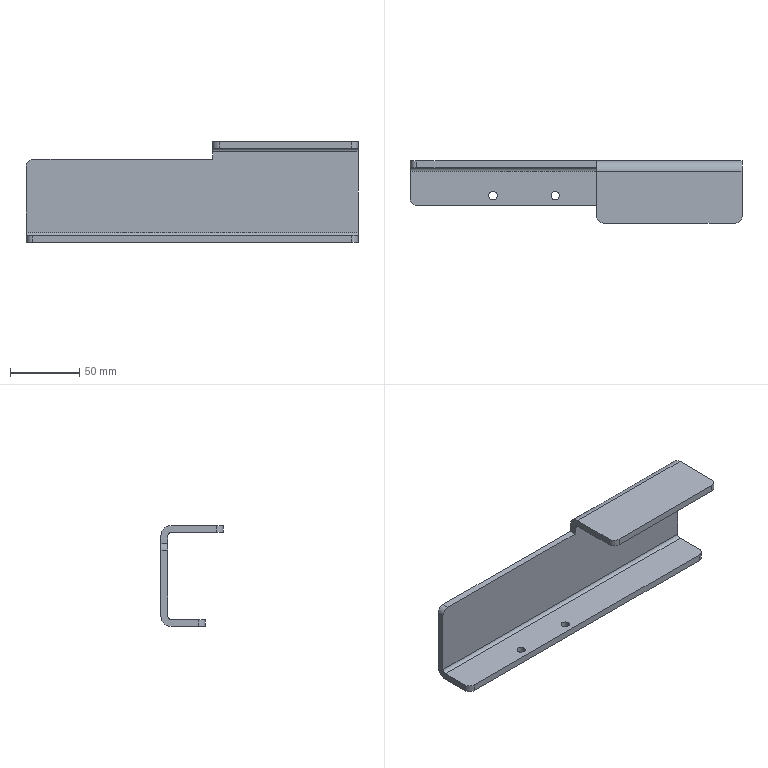Part | NX | 1 solid | 29 faces | box 240 x 45 x 73 mm | volume 128180 mm3 | cylinder 13 | plane 12 | cone 4 | commonest cylinder face diameters 10 x5 6 x4 4.8 x2 14.8 x2
STEP:
#1=CARTESIAN_POINT('',(2327.5,238.4,-44.7));
#2=VERTEX_POINT('',#1);
#3=CARTESIAN_POINT('',(2327.5,238.4,-49.7));
#4=VERTEX_POINT('',#3);
#5=CARTESIAN_POINT('',(2327.5,238.4,-49.7));
#6=DIRECTION('',(0.,0.,-1.));
#7=VECTOR('',#6,1000.);
#8=LINE('',#5,#7);
#9=EDGE_CURVE('',#2,#4,#8,.T.);
#10=ORIENTED_EDGE('',*,*,#9,.F.);
#11=CARTESIAN_POINT('',(2097.5,238.4,-44.7));
#12=VERTEX_POINT('',#11);
#13=CARTESIAN_POINT('',(2161.418,238.4,-44.7));
#14=DIRECTION('',(-1.,0.,0.));
#15=VECTOR('',#14,1000.);
#16=LINE('',#13,#15);
#17=EDGE_CURVE('',#2,#12,#16,.T.);
#18=ORIENTED_EDGE('',*,*,#17,.T.);
#19=CARTESIAN_POINT('',(2097.5,238.4,-49.7));
#20=VERTEX_POINT('',#19);
#21=CARTESIAN_POINT('',(2097.5,238.4,-49.7));
#22=DIRECTION('',(0.,0.,1.));
#23=VECTOR('',#22,1000.);
#24=LINE('',#21,#23);
#25=EDGE_CURVE('',#20,#12,#24,.T.);
#26=ORIENTED_EDGE('',*,*,#25,.F.);
#27=CARTESIAN_POINT('',(2161.418,238.4,-49.7));
#28=DIRECTION('',(-1.,0.,0.));
#29=VECTOR('',#28,1000.);
#30=LINE('',#27,#29);
#31=EDGE_CURVE('',#4,#20,#30,.T.);
#32=ORIENTED_EDGE('',*,*,#31,.F.);
#33=EDGE_LOOP('',(#10,#18,#26,#32));
#34=FACE_BOUND('',#33,.T.);
#35=CARTESIAN_POINT('',(2227.5,238.4,-49.7));
#36=DIRECTION('',(0.,-1.,0.));
#37=DIRECTION('',(0.,0.,-1.));
#38=AXIS2_PLACEMENT_3D('',#35,#36,#37);
#39=PLANE('',#38);
#40=ADVANCED_FACE('',(#34),#39,.T.);
#41=ORIENTED_EDGE('',*,*,#9,.T.);
#42=CARTESIAN_POINT('',(2332.5,243.4,-49.7));
#43=VERTEX_POINT('',#42);
#44=CARTESIAN_POINT('',(2327.5,243.4,-49.7));
#45=DIRECTION('',(0.,0.,-1.));
#46=DIRECTION('',(-1.,0.,0.));
#47=AXIS2_PLACEMENT_3D('',#44,#45,#46);
#48=CIRCLE('',#47,5.);
#49=EDGE_CURVE('',#43,#4,#48,.T.);
#50=ORIENTED_EDGE('',*,*,#49,.F.);
#51=CARTESIAN_POINT('',(2332.5,243.4,-44.7));
#52=VERTEX_POINT('',#51);
#53=CARTESIAN_POINT('',(2332.5,243.4,-49.7));
#54=DIRECTION('',(0.,0.,-1.));
#55=VECTOR('',#54,1000.);
#56=LINE('',#53,#55);
#57=EDGE_CURVE('',#52,#43,#56,.T.);
#58=ORIENTED_EDGE('',*,*,#57,.F.);
#59=CARTESIAN_POINT('',(2327.5,243.4,-44.7));
#60=DIRECTION('',(0.,0.,-1.));
#61=DIRECTION('',(-1.,0.,0.));
#62=AXIS2_PLACEMENT_3D('',#59,#60,#61);
#63=CIRCLE('',#62,5.);
#64=EDGE_CURVE('',#52,#2,#63,.T.);
#65=ORIENTED_EDGE('',*,*,#64,.T.);
#66=EDGE_LOOP('',(#41,#50,#58,#65));
#67=FACE_BOUND('',#66,.T.);
#68=CARTESIAN_POINT('',(2327.5,243.4,-49.7));
#69=DIRECTION('',(0.,0.,-1.));
#70=DIRECTION('',(-1.,0.,0.));
#71=AXIS2_PLACEMENT_3D('',#68,#69,#70);
#72=CYLINDRICAL_SURFACE('',#71,5.);
#73=ADVANCED_FACE('',(#67),#72,.T.);
#74=CARTESIAN_POINT('',(2200.5,245.4,-49.5));
#75=VERTEX_POINT('',#74);
#76=CARTESIAN_POINT('',(2194.5,245.4,-49.5));
#77=VERTEX_POINT('',#76);
#78=CARTESIAN_POINT('',(2197.5,245.4,-49.5));
#79=DIRECTION('',(0.,0.,-1.));
#80=DIRECTION('',(-1.,0.,0.));
#81=AXIS2_PLACEMENT_3D('',#78,#79,#80);
#82=CIRCLE('',#81,3.);
#83=EDGE_CURVE('',#75,#77,#82,.T.);
#84=ORIENTED_EDGE('',*,*,#83,.T.);
#85=CARTESIAN_POINT('',(2194.5,245.4,-44.7));
#86=VERTEX_POINT('',#85);
#87=CARTESIAN_POINT('',(2194.5,245.4,-49.7));
#88=DIRECTION('',(0.,0.,-1.));
#89=VECTOR('',#88,1000.);
#90=LINE('',#87,#89);
#91=EDGE_CURVE('',#77,#86,#90,.F.);
#92=ORIENTED_EDGE('',*,*,#91,.T.);
#93=CARTESIAN_POINT('',(2200.5,245.4,-44.7));
#94=VERTEX_POINT('',#93);
#95=CARTESIAN_POINT('',(2197.5,245.4,-44.7));
#96=DIRECTION('',(0.,0.,-1.));
#97=DIRECTION('',(-1.,0.,0.));
#98=AXIS2_PLACEMENT_3D('',#95,#96,#97);
#99=CIRCLE('',#98,3.);
#100=EDGE_CURVE('',#94,#86,#99,.T.);
#101=ORIENTED_EDGE('',*,*,#100,.F.);
#102=CARTESIAN_POINT('',(2200.5,245.4,-49.7));
#103=DIRECTION('',(0.,0.,-1.));
#104=VECTOR('',#103,1000.);
#105=LINE('',#102,#104);
#106=EDGE_CURVE('',#75,#94,#105,.F.);
#107=ORIENTED_EDGE('',*,*,#106,.F.);
#108=EDGE_LOOP('',(#84,#92,#101,#107));
#109=FACE_BOUND('',#108,.T.);
#110=CARTESIAN_POINT('',(2197.5,245.4,-49.7));
#111=DIRECTION('',(0.,0.,-1.));
#112=DIRECTION('',(-1.,0.,0.));
#113=AXIS2_PLACEMENT_3D('',#110,#111,#112);
#114=CYLINDRICAL_SURFACE('',#113,3.);
#115=ADVANCED_FACE('',(#109),#114,.F.);
#116=ORIENTED_EDGE('',*,*,#83,.F.);
#117=CARTESIAN_POINT('',(2200.7,245.4,-49.7));
#118=VERTEX_POINT('',#117);
#119=CARTESIAN_POINT('',(2200.5,245.4,-49.5));
#120=DIRECTION('',(0.7071,0.,-0.7071));
#121=VECTOR('',#120,1000.);
#122=LINE('',#119,#121);
#123=EDGE_CURVE('',#118,#75,#122,.F.);
#124=ORIENTED_EDGE('',*,*,#123,.F.);
#125=CARTESIAN_POINT('',(2194.3,245.4,-49.7));
#126=VERTEX_POINT('',#125);
#127=CARTESIAN_POINT('',(2197.5,245.4,-49.7));
#128=DIRECTION('',(0.,0.,-1.));
#129=DIRECTION('',(-1.,0.,0.));
#130=AXIS2_PLACEMENT_3D('',#127,#128,#129);
#131=CIRCLE('',#130,3.2);
#132=EDGE_CURVE('',#118,#126,#131,.T.);
#133=ORIENTED_EDGE('',*,*,#132,.T.);
#134=CARTESIAN_POINT('',(2194.5,245.4,-49.5));
#135=DIRECTION('',(-0.7071,0.,-0.7071));
#136=VECTOR('',#135,1000.);
#137=LINE('',#134,#136);
#138=EDGE_CURVE('',#126,#77,#137,.F.);
#139=ORIENTED_EDGE('',*,*,#138,.T.);
#140=EDGE_LOOP('',(#116,#124,#133,#139));
#141=FACE_BOUND('',#140,.T.);
#142=CARTESIAN_POINT('',(2197.5,245.4,-49.5));
#143=DIRECTION('',(0.,0.,-1.));
#144=DIRECTION('',(-1.,0.,0.));
#145=AXIS2_PLACEMENT_3D('',#142,#143,#144);
#146=CONICAL_SURFACE('',#145,3.,0.7854);
#147=ADVANCED_FACE('',(#141),#146,.F.);
#148=ORIENTED_EDGE('',*,*,#91,.F.);
#149=CARTESIAN_POINT('',(2197.5,245.4,-49.5));
#150=DIRECTION('',(0.,0.,-1.));
#151=DIRECTION('',(-1.,0.,0.));
#152=AXIS2_PLACEMENT_3D('',#149,#150,#151);
#153=CIRCLE('',#152,3.);
#154=EDGE_CURVE('',#77,#75,#153,.T.);
#155=ORIENTED_EDGE('',*,*,#154,.T.);
#156=ORIENTED_EDGE('',*,*,#106,.T.);
#157=CARTESIAN_POINT('',(2197.5,245.4,-44.7));
#158=DIRECTION('',(0.,0.,-1.));
#159=DIRECTION('',(-1.,0.,0.));
#160=AXIS2_PLACEMENT_3D('',#157,#158,#159);
#161=CIRCLE('',#160,3.);
#162=EDGE_CURVE('',#86,#94,#161,.T.);
#163=ORIENTED_EDGE('',*,*,#162,.F.);
#164=EDGE_LOOP('',(#148,#155,#156,#163));
#165=FACE_BOUND('',#164,.T.);
#166=CARTESIAN_POINT('',(2197.5,245.4,-49.7));
#167=DIRECTION('',(0.,0.,-1.));
#168=DIRECTION('',(-1.,0.,0.));
#169=AXIS2_PLACEMENT_3D('',#166,#167,#168);
#170=CYLINDRICAL_SURFACE('',#169,3.);
#171=ADVANCED_FACE('',(#165),#170,.F.);
#172=ORIENTED_EDGE('',*,*,#138,.F.);
#173=CARTESIAN_POINT('',(2197.5,245.4,-49.7));
#174=DIRECTION('',(0.,0.,-1.));
#175=DIRECTION('',(-1.,0.,0.));
#176=AXIS2_PLACEMENT_3D('',#173,#174,#175);
#177=CIRCLE('',#176,3.2);
#178=EDGE_CURVE('',#126,#118,#177,.T.);
#179=ORIENTED_EDGE('',*,*,#178,.T.);
#180=ORIENTED_EDGE('',*,*,#123,.T.);
#181=ORIENTED_EDGE('',*,*,#154,.F.);
#182=EDGE_LOOP('',(#172,#179,#180,#181));
#183=FACE_BOUND('',#182,.T.);
#184=CARTESIAN_POINT('',(2197.5,245.4,-49.5));
#185=DIRECTION('',(0.,0.,-1.));
#186=DIRECTION('',(-1.,0.,0.));
#187=AXIS2_PLACEMENT_3D('',#184,#185,#186);
#188=CONICAL_SURFACE('',#187,3.,0.7854);
#189=ADVANCED_FACE('',(#183),#188,.F.);
#190=CARTESIAN_POINT('',(2092.5,263.,-44.7));
#191=VERTEX_POINT('',#190);
#192=CARTESIAN_POINT('',(2092.5,243.4,-44.7));
#193=VERTEX_POINT('',#192);
#194=CARTESIAN_POINT('',(2092.5,301.297,-44.7));
#195=DIRECTION('',(0.,-1.,0.));
#196=VECTOR('',#195,1000.);
#197=LINE('',#194,#196);
#198=EDGE_CURVE('',#191,#193,#197,.T.);
#199=ORIENTED_EDGE('',*,*,#198,.T.);
#200=CARTESIAN_POINT('',(2097.5,243.4,-44.7));
#201=DIRECTION('',(0.,0.,1.));
#202=DIRECTION('',(1.,0.,0.));
#203=AXIS2_PLACEMENT_3D('',#200,#201,#202);
#204=CIRCLE('',#203,5.);
#205=EDGE_CURVE('',#193,#12,#204,.T.);
#206=ORIENTED_EDGE('',*,*,#205,.T.);
#207=ORIENTED_EDGE('',*,*,#17,.F.);
#208=ORIENTED_EDGE('',*,*,#64,.F.);
#209=CARTESIAN_POINT('',(2332.5,263.,-44.7));
#210=VERTEX_POINT('',#209);
#211=CARTESIAN_POINT('',(2332.5,249.699,-44.7));
#212=DIRECTION('',(0.,1.,0.));
#213=VECTOR('',#212,1000.);
#214=LINE('',#211,#213);
#215=EDGE_CURVE('',#52,#210,#214,.T.);
#216=ORIENTED_EDGE('',*,*,#215,.T.);
#217=CARTESIAN_POINT('',(2161.418,263.,-44.7));
#218=DIRECTION('',(-1.,0.,0.));
#219=VECTOR('',#218,1000.);
#220=LINE('',#217,#219);
#221=EDGE_CURVE('',#210,#191,#220,.T.);
#222=ORIENTED_EDGE('',*,*,#221,.T.);
#223=EDGE_LOOP('',(#199,#206,#207,#208,#216,#222));
#224=FACE_BOUND('',#223,.T.);
#225=CARTESIAN_POINT('',(2155.5,245.4,-44.7));
#226=VERTEX_POINT('',#225);
#227=CARTESIAN_POINT('',(2149.5,245.4,-44.7));
#228=VERTEX_POINT('',#227);
#229=CARTESIAN_POINT('',(2152.5,245.4,-44.7));
#230=DIRECTION('',(0.,0.,-1.));
#231=DIRECTION('',(-1.,0.,0.));
#232=AXIS2_PLACEMENT_3D('',#229,#230,#231);
#233=CIRCLE('',#232,3.);
#234=EDGE_CURVE('',#226,#228,#233,.T.);
#235=ORIENTED_EDGE('',*,*,#234,.T.);
#236=CARTESIAN_POINT('',(2152.5,245.4,-44.7));
#237=DIRECTION('',(0.,0.,-1.));
#238=DIRECTION('',(-1.,0.,0.));
#239=AXIS2_PLACEMENT_3D('',#236,#237,#238);
#240=CIRCLE('',#239,3.);
#241=EDGE_CURVE('',#228,#226,#240,.T.);
#242=ORIENTED_EDGE('',*,*,#241,.T.);
#243=EDGE_LOOP('',(#235,#242));
#244=FACE_BOUND('',#243,.T.);
#245=ORIENTED_EDGE('',*,*,#100,.T.);
#246=ORIENTED_EDGE('',*,*,#162,.T.);
#247=EDGE_LOOP('',(#245,#246));
#248=FACE_BOUND('',#247,.T.);
#249=CARTESIAN_POINT('',(2161.418,249.699,-44.7));
#250=DIRECTION('',(0.,0.,-1.));
#251=DIRECTION('',(-1.,0.,0.));
#252=AXIS2_PLACEMENT_3D('',#249,#250,#251);
#253=PLANE('',#252);
#254=ADVANCED_FACE('',(#224,#244,#248),#253,.F.);
#255=ORIENTED_EDGE('',*,*,#221,.F.);
#256=CARTESIAN_POINT('',(2332.5,265.4,-42.3));
#257=VERTEX_POINT('',#256);
#258=CARTESIAN_POINT('',(2332.5,263.,-42.3));
#259=DIRECTION('',(-1.,0.,0.));
#260=DIRECTION('',(0.,-1.,0.));
#261=AXIS2_PLACEMENT_3D('',#258,#259,#260);
#262=CIRCLE('',#261,2.4);
#263=EDGE_CURVE('',#257,#210,#262,.T.);
#264=ORIENTED_EDGE('',*,*,#263,.F.);
#265=CARTESIAN_POINT('',(2092.5,265.4,-42.3));
#266=VERTEX_POINT('',#265);
#267=CARTESIAN_POINT('',(2161.418,265.4,-42.3));
#268=DIRECTION('',(-1.,0.,0.));
#269=VECTOR('',#268,1000.);
#270=LINE('',#267,#269);
#271=EDGE_CURVE('',#257,#266,#270,.T.);
#272=ORIENTED_EDGE('',*,*,#271,.T.);
#273=CARTESIAN_POINT('',(2092.5,263.,-42.3));
#274=DIRECTION('',(-1.,0.,0.));
#275=DIRECTION('',(0.,1.,0.));
#276=AXIS2_PLACEMENT_3D('',#273,#274,#275);
#277=CIRCLE('',#276,2.4);
#278=EDGE_CURVE('',#266,#191,#277,.T.);
#279=ORIENTED_EDGE('',*,*,#278,.T.);
#280=EDGE_LOOP('',(#255,#264,#272,#279));
#281=FACE_BOUND('',#280,.T.);
#282=CARTESIAN_POINT('',(2092.5,263.,-42.3));
#283=DIRECTION('',(-1.,0.,0.));
#284=DIRECTION('',(0.,-1.,0.));
#285=AXIS2_PLACEMENT_3D('',#282,#283,#284);
#286=CYLINDRICAL_SURFACE('',#285,2.4);
#287=ADVANCED_FACE('',(#281),#286,.F.);
#288=ORIENTED_EDGE('',*,*,#271,.F.);
#289=CARTESIAN_POINT('',(2332.5,265.4,15.9));
#290=VERTEX_POINT('',#289);
#291=CARTESIAN_POINT('',(2332.5,265.4,-49.7));
#292=DIRECTION('',(0.,0.,1.));
#293=VECTOR('',#292,1000.);
#294=LINE('',#291,#293);
#295=EDGE_CURVE('',#257,#290,#294,.T.);
#296=ORIENTED_EDGE('',*,*,#295,.T.);
#297=CARTESIAN_POINT('',(2227.5,265.4,15.9));
#298=VERTEX_POINT('',#297);
#299=CARTESIAN_POINT('',(2161.418,265.4,15.9));
#300=DIRECTION('',(-1.,0.,0.));
#301=VECTOR('',#300,1000.);
#302=LINE('',#299,#301);
#303=EDGE_CURVE('',#290,#298,#302,.T.);
#304=ORIENTED_EDGE('',*,*,#303,.T.);
#305=CARTESIAN_POINT('',(2227.5,265.4,10.3));
#306=VERTEX_POINT('',#305);
#307=CARTESIAN_POINT('',(2227.5,265.4,39.197));
#308=DIRECTION('',(0.,0.,-1.));
#309=VECTOR('',#308,1000.);
#310=LINE('',#307,#309);
#311=EDGE_CURVE('',#298,#306,#310,.T.);
#312=ORIENTED_EDGE('',*,*,#311,.T.);
#313=CARTESIAN_POINT('',(2097.5,265.4,10.3));
#314=VERTEX_POINT('',#313);
#315=CARTESIAN_POINT('',(2161.418,265.4,10.3));
#316=DIRECTION('',(1.,0.,0.));
#317=VECTOR('',#316,1000.);
#318=LINE('',#315,#317);
#319=EDGE_CURVE('',#314,#306,#318,.T.);
#320=ORIENTED_EDGE('',*,*,#319,.F.);
#321=CARTESIAN_POINT('',(2092.5,265.4,5.3));
#322=VERTEX_POINT('',#321);
#323=CARTESIAN_POINT('',(2097.5,265.4,5.3));
#324=DIRECTION('',(0.,1.,0.));
#325=DIRECTION('',(0.,0.,1.));
#326=AXIS2_PLACEMENT_3D('',#323,#324,#325);
#327=CIRCLE('',#326,5.);
#328=EDGE_CURVE('',#322,#314,#327,.T.);
#329=ORIENTED_EDGE('',*,*,#328,.F.);
#330=CARTESIAN_POINT('',(2092.5,265.4,-49.7));
#331=DIRECTION('',(0.,0.,-1.));
#332=VECTOR('',#331,1000.);
#333=LINE('',#330,#332);
#334=EDGE_CURVE('',#322,#266,#333,.T.);
#335=ORIENTED_EDGE('',*,*,#334,.T.);
#336=EDGE_LOOP('',(#288,#296,#304,#312,#320,#329,#335));
#337=FACE_BOUND('',#336,.T.);
#338=CARTESIAN_POINT('',(2161.418,265.4,-61.297));
#339=DIRECTION('',(0.,1.,0.));
#340=DIRECTION('',(0.,0.,-1.));
#341=AXIS2_PLACEMENT_3D('',#338,#339,#340);
#342=PLANE('',#341);
#343=ADVANCED_FACE('',(#337),#342,.F.);
#344=CARTESIAN_POINT('',(2097.5,270.4,10.3));
#345=VERTEX_POINT('',#344);
#346=CARTESIAN_POINT('',(2097.5,249.699,10.3));
#347=DIRECTION('',(0.,1.,0.));
#348=VECTOR('',#347,1000.);
#349=LINE('',#346,#348);
#350=EDGE_CURVE('',#314,#345,#349,.T.);
#351=ORIENTED_EDGE('',*,*,#350,.F.);
#352=ORIENTED_EDGE('',*,*,#319,.T.);
#353=CARTESIAN_POINT('',(2227.5,270.4,10.3));
#354=VERTEX_POINT('',#353);
#355=CARTESIAN_POINT('',(2227.5,270.4,10.3));
#356=DIRECTION('',(0.,-1.,0.));
#357=VECTOR('',#356,1000.);
#358=LINE('',#355,#357);
#359=EDGE_CURVE('',#354,#306,#358,.T.);
#360=ORIENTED_EDGE('',*,*,#359,.F.);
#361=CARTESIAN_POINT('',(2161.418,270.4,10.3));
#362=DIRECTION('',(1.,0.,0.));
#363=VECTOR('',#362,1000.);
#364=LINE('',#361,#363);
#365=EDGE_CURVE('',#345,#354,#364,.T.);
#366=ORIENTED_EDGE('',*,*,#365,.F.);
#367=EDGE_LOOP('',(#351,#352,#360,#366));
#368=FACE_BOUND('',#367,.T.);
#369=CARTESIAN_POINT('',(2319.141,266.915,10.3));
#370=DIRECTION('',(0.,0.,1.));
#371=DIRECTION('',(1.,0.,0.));
#372=AXIS2_PLACEMENT_3D('',#369,#370,#371);
#373=PLANE('',#372);
#374=ADVANCED_FACE('',(#368),#373,.T.);
#375=ORIENTED_EDGE('',*,*,#303,.F.);
#376=CARTESIAN_POINT('',(2332.5,263.,18.3));
#377=VERTEX_POINT('',#376);
#378=CARTESIAN_POINT('',(2332.5,263.,15.9));
#379=DIRECTION('',(-1.,0.,0.));
#380=DIRECTION('',(0.,-1.,0.));
#381=AXIS2_PLACEMENT_3D('',#378,#379,#380);
#382=CIRCLE('',#381,2.4);
#383=EDGE_CURVE('',#377,#290,#382,.T.);
#384=ORIENTED_EDGE('',*,*,#383,.F.);
#385=CARTESIAN_POINT('',(2227.5,263.,18.3));
#386=VERTEX_POINT('',#385);
#387=CARTESIAN_POINT('',(2161.418,263.,18.3));
#388=DIRECTION('',(-1.,0.,0.));
#389=VECTOR('',#388,1000.);
#390=LINE('',#387,#389);
#391=EDGE_CURVE('',#377,#386,#390,.T.);
#392=ORIENTED_EDGE('',*,*,#391,.T.);
#393=CARTESIAN_POINT('',(2227.5,263.,15.9));
#394=DIRECTION('',(-1.,0.,0.));
#395=DIRECTION('',(0.,0.,1.));
#396=AXIS2_PLACEMENT_3D('',#393,#394,#395);
#397=CIRCLE('',#396,2.4);
#398=EDGE_CURVE('',#386,#298,#397,.T.);
#399=ORIENTED_EDGE('',*,*,#398,.T.);
#400=EDGE_LOOP('',(#375,#384,#392,#399));
#401=FACE_BOUND('',#400,.T.);
#402=CARTESIAN_POINT('',(2227.5,263.,15.9));
#403=DIRECTION('',(-1.,0.,0.));
#404=DIRECTION('',(0.,-1.,0.));
#405=AXIS2_PLACEMENT_3D('',#402,#403,#404);
#406=CYLINDRICAL_SURFACE('',#405,2.4);
#407=ADVANCED_FACE('',(#401),#406,.F.);
#408=ORIENTED_EDGE('',*,*,#391,.F.);
#409=CARTESIAN_POINT('',(2332.5,230.4,18.3));
#410=VERTEX_POINT('',#409);
#411=CARTESIAN_POINT('',(2332.5,249.699,18.3));
#412=DIRECTION('',(0.,-1.,0.));
#413=VECTOR('',#412,1000.);
#414=LINE('',#411,#413);
#415=EDGE_CURVE('',#377,#410,#414,.T.);
#416=ORIENTED_EDGE('',*,*,#415,.T.);
#417=CARTESIAN_POINT('',(2327.5,225.4,18.3));
#418=VERTEX_POINT('',#417);
#419=CARTESIAN_POINT('',(2327.5,230.4,18.3));
#420=DIRECTION('',(0.,0.,1.));
#421=DIRECTION('',(1.,0.,0.));
#422=AXIS2_PLACEMENT_3D('',#419,#420,#421);
#423=CIRCLE('',#422,5.);
#424=EDGE_CURVE('',#418,#410,#423,.T.);
#425=ORIENTED_EDGE('',*,*,#424,.F.);
#426=CARTESIAN_POINT('',(2232.5,225.4,18.3));
#427=VERTEX_POINT('',#426);
#428=CARTESIAN_POINT('',(2161.418,225.4,18.3));
#429=DIRECTION('',(1.,0.,0.));
#430=VECTOR('',#429,1000.);
#431=LINE('',#428,#430);
#432=EDGE_CURVE('',#427,#418,#431,.T.);
#433=ORIENTED_EDGE('',*,*,#432,.F.);
#434=CARTESIAN_POINT('',(2227.5,230.4,18.3));
#435=VERTEX_POINT('',#434);
#436=CARTESIAN_POINT('',(2232.5,230.4,18.3));
#437=DIRECTION('',(0.,0.,1.));
#438=DIRECTION('',(1.,0.,0.));
#439=AXIS2_PLACEMENT_3D('',#436,#437,#438);
#440=CIRCLE('',#439,5.);
#441=EDGE_CURVE('',#435,#427,#440,.T.);
#442=ORIENTED_EDGE('',*,*,#441,.F.);
#443=CARTESIAN_POINT('',(2227.5,249.699,18.3));
#444=DIRECTION('',(0.,1.,0.));
#445=VECTOR('',#444,1000.);
#446=LINE('',#443,#445);
#447=EDGE_CURVE('',#435,#386,#446,.T.);
#448=ORIENTED_EDGE('',*,*,#447,.T.);
#449=EDGE_LOOP('',(#408,#416,#425,#433,#442,#448));
#450=FACE_BOUND('',#449,.T.);
#451=CARTESIAN_POINT('',(2161.418,345.894,18.3));
#452=DIRECTION('',(0.,0.,1.));
#453=DIRECTION('',(0.,-1.,0.));
#454=AXIS2_PLACEMENT_3D('',#451,#452,#453);
#455=PLANE('',#454);
#456=ADVANCED_FACE('',(#450),#455,.F.);
#457=ORIENTED_EDGE('',*,*,#350,.T.);
#458=CARTESIAN_POINT('',(2092.5,270.4,5.3));
#459=VERTEX_POINT('',#458);
#460=CARTESIAN_POINT('',(2097.5,270.4,5.3));
#461=DIRECTION('',(0.,1.,0.));
#462=DIRECTION('',(0.,0.,1.));
#463=AXIS2_PLACEMENT_3D('',#460,#461,#462);
#464=CIRCLE('',#463,5.);
#465=EDGE_CURVE('',#459,#345,#464,.T.);
#466=ORIENTED_EDGE('',*,*,#465,.F.);
#467=CARTESIAN_POINT('',(2092.5,249.699,5.3));
#468=DIRECTION('',(0.,1.,0.));
#469=VECTOR('',#468,1000.);
#470=LINE('',#467,#469);
#471=EDGE_CURVE('',#322,#459,#470,.T.);
#472=ORIENTED_EDGE('',*,*,#471,.F.);
#473=ORIENTED_EDGE('',*,*,#328,.T.);
#474=EDGE_LOOP('',(#457,#466,#472,#473));
#475=FACE_BOUND('',#474,.T.);
#476=CARTESIAN_POINT('',(2097.5,249.699,5.3));
#477=DIRECTION('',(0.,1.,0.));
#478=DIRECTION('',(0.,0.,1.));
#479=AXIS2_PLACEMENT_3D('',#476,#477,#478);
#480=CYLINDRICAL_SURFACE('',#479,5.);
#481=ADVANCED_FACE('',(#475),#480,.T.);
#482=CARTESIAN_POINT('',(2155.5,245.4,-49.5));
#483=VERTEX_POINT('',#482);
#484=CARTESIAN_POINT('',(2149.5,245.4,-49.5));
#485=VERTEX_POINT('',#484);
#486=CARTESIAN_POINT('',(2152.5,245.4,-49.5));
#487=DIRECTION('',(0.,0.,-1.));
#488=DIRECTION('',(-1.,0.,0.));
#489=AXIS2_PLACEMENT_3D('',#486,#487,#488);
#490=CIRCLE('',#489,3.);
#491=EDGE_CURVE('',#483,#485,#490,.T.);
#492=ORIENTED_EDGE('',*,*,#491,.T.);
#493=CARTESIAN_POINT('',(2149.5,245.4,-49.7));
#494=DIRECTION('',(0.,0.,-1.));
#495=VECTOR('',#494,1000.);
#496=LINE('',#493,#495);
#497=EDGE_CURVE('',#485,#228,#496,.F.);
#498=ORIENTED_EDGE('',*,*,#497,.T.);
#499=ORIENTED_EDGE('',*,*,#234,.F.);
#500=CARTESIAN_POINT('',(2155.5,245.4,-49.7));
#501=DIRECTION('',(0.,0.,-1.));
#502=VECTOR('',#501,1000.);
#503=LINE('',#500,#502);
#504=EDGE_CURVE('',#483,#226,#503,.F.);
#505=ORIENTED_EDGE('',*,*,#504,.F.);
#506=EDGE_LOOP('',(#492,#498,#499,#505));
#507=FACE_BOUND('',#506,.T.);
#508=CARTESIAN_POINT('',(2152.5,245.4,-49.7));
#509=DIRECTION('',(0.,0.,-1.));
#510=DIRECTION('',(-1.,0.,0.));
#511=AXIS2_PLACEMENT_3D('',#508,#509,#510);
#512=CYLINDRICAL_SURFACE('',#511,3.);
#513=ADVANCED_FACE('',(#507),#512,.F.);
#514=ORIENTED_EDGE('',*,*,#491,.F.);
#515=CARTESIAN_POINT('',(2155.7,245.4,-49.7));
#516=VERTEX_POINT('',#515);
#517=CARTESIAN_POINT('',(2155.5,245.4,-49.5));
#518=DIRECTION('',(0.7071,0.,-0.7071));
#519=VECTOR('',#518,1000.);
#520=LINE('',#517,#519);
#521=EDGE_CURVE('',#516,#483,#520,.F.);
#522=ORIENTED_EDGE('',*,*,#521,.F.);
#523=CARTESIAN_POINT('',(2149.3,245.4,-49.7));
#524=VERTEX_POINT('',#523);
#525=CARTESIAN_POINT('',(2152.5,245.4,-49.7));
#526=DIRECTION('',(0.,0.,-1.));
#527=DIRECTION('',(-1.,0.,0.));
#528=AXIS2_PLACEMENT_3D('',#525,#526,#527);
#529=CIRCLE('',#528,3.2);
#530=EDGE_CURVE('',#516,#524,#529,.T.);
#531=ORIENTED_EDGE('',*,*,#530,.T.);
#532=CARTESIAN_POINT('',(2149.5,245.4,-49.5));
#533=DIRECTION('',(-0.7071,0.,-0.7071));
#534=VECTOR('',#533,1000.);
#535=LINE('',#532,#534);
#536=EDGE_CURVE('',#524,#485,#535,.F.);
#537=ORIENTED_EDGE('',*,*,#536,.T.);
#538=EDGE_LOOP('',(#514,#522,#531,#537));
#539=FACE_BOUND('',#538,.T.);
#540=CARTESIAN_POINT('',(2152.5,245.4,-49.5));
#541=DIRECTION('',(0.,0.,-1.));
#542=DIRECTION('',(-1.,0.,0.));
#543=AXIS2_PLACEMENT_3D('',#540,#541,#542);
#544=CONICAL_SURFACE('',#543,3.,0.7854);
#545=ADVANCED_FACE('',(#539),#544,.F.);
#546=ORIENTED_EDGE('',*,*,#497,.F.);
#547=CARTESIAN_POINT('',(2152.5,245.4,-49.5));
#548=DIRECTION('',(0.,0.,-1.));
#549=DIRECTION('',(-1.,0.,0.));
#550=AXIS2_PLACEMENT_3D('',#547,#548,#549);
#551=CIRCLE('',#550,3.);
#552=EDGE_CURVE('',#485,#483,#551,.T.);
#553=ORIENTED_EDGE('',*,*,#552,.T.);
#554=ORIENTED_EDGE('',*,*,#504,.T.);
#555=ORIENTED_EDGE('',*,*,#241,.F.);
#556=EDGE_LOOP('',(#546,#553,#554,#555));
#557=FACE_BOUND('',#556,.T.);
#558=CARTESIAN_POINT('',(2152.5,245.4,-49.7));
#559=DIRECTION('',(0.,0.,-1.));
#560=DIRECTION('',(-1.,0.,0.));
#561=AXIS2_PLACEMENT_3D('',#558,#559,#560);
#562=CYLINDRICAL_SURFACE('',#561,3.);
#563=ADVANCED_FACE('',(#557),#562,.F.);
#564=ORIENTED_EDGE('',*,*,#536,.F.);
#565=CARTESIAN_POINT('',(2152.5,245.4,-49.7));
#566=DIRECTION('',(0.,0.,-1.));
#567=DIRECTION('',(-1.,0.,0.));
#568=AXIS2_PLACEMENT_3D('',#565,#566,#567);
#569=CIRCLE('',#568,3.2);
#570=EDGE_CURVE('',#524,#516,#569,.T.);
#571=ORIENTED_EDGE('',*,*,#570,.T.);
#572=ORIENTED_EDGE('',*,*,#521,.T.);
#573=ORIENTED_EDGE('',*,*,#552,.F.);
#574=EDGE_LOOP('',(#564,#571,#572,#573));
#575=FACE_BOUND('',#574,.T.);
#576=CARTESIAN_POINT('',(2152.5,245.4,-49.5));
#577=DIRECTION('',(0.,0.,-1.));
#578=DIRECTION('',(-1.,0.,0.));
#579=AXIS2_PLACEMENT_3D('',#576,#577,#578);
#580=CONICAL_SURFACE('',#579,3.,0.7854);
#581=ADVANCED_FACE('',(#575),#580,.F.);
#582=CARTESIAN_POINT('',(2092.5,243.4,-49.7));
#583=VERTEX_POINT('',#582);
#584=CARTESIAN_POINT('',(2092.5,243.4,-49.7));
#585=DIRECTION('',(0.,0.,1.));
#586=VECTOR('',#585,1000.);
#587=LINE('',#584,#586);
#588=EDGE_CURVE('',#583,#193,#587,.T.);
#589=ORIENTED_EDGE('',*,*,#588,.T.);
#590=ORIENTED_EDGE('',*,*,#198,.F.);
#591=ORIENTED_EDGE('',*,*,#278,.F.);
#592=ORIENTED_EDGE('',*,*,#334,.F.);
#593=ORIENTED_EDGE('',*,*,#471,.T.);
#594=CARTESIAN_POINT('',(2092.5,270.4,-42.3));
#595=VERTEX_POINT('',#594);
#596=CARTESIAN_POINT('',(2092.5,270.4,-49.7));
#597=DIRECTION('',(0.,0.,-1.));
#598=VECTOR('',#597,1000.);
#599=LINE('',#596,#598);
#600=EDGE_CURVE('',#459,#595,#599,.T.);
#601=ORIENTED_EDGE('',*,*,#600,.T.);
#602=CARTESIAN_POINT('',(2092.5,263.,-49.7));
#603=VERTEX_POINT('',#602);
#604=CARTESIAN_POINT('',(2092.5,263.,-42.3));
#605=DIRECTION('',(-1.,0.,0.));
#606=DIRECTION('',(0.,1.,0.));
#607=AXIS2_PLACEMENT_3D('',#604,#605,#606);
#608=CIRCLE('',#607,7.4);
#609=EDGE_CURVE('',#595,#603,#608,.T.);
#610=ORIENTED_EDGE('',*,*,#609,.T.);
#611=CARTESIAN_POINT('',(2092.5,249.699,-49.7));
#612=DIRECTION('',(0.,-1.,0.));
#613=VECTOR('',#612,1000.);
#614=LINE('',#611,#613);
#615=EDGE_CURVE('',#603,#583,#614,.T.);
#616=ORIENTED_EDGE('',*,*,#615,.T.);
#617=EDGE_LOOP('',(#589,#590,#591,#592,#593,#601,#610,#616));
#618=FACE_BOUND('',#617,.T.);
#619=CARTESIAN_POINT('',(2092.5,270.4,-49.7));
#620=DIRECTION('',(-1.,0.,0.));
#621=DIRECTION('',(0.,0.,1.));
#622=AXIS2_PLACEMENT_3D('',#619,#620,#621);
#623=PLANE('',#622);
#624=ADVANCED_FACE('',(#618),#623,.T.);
#625=CARTESIAN_POINT('',(2332.5,230.4,23.3));
#626=VERTEX_POINT('',#625);
#627=CARTESIAN_POINT('',(2332.5,230.4,-49.7));
#628=DIRECTION('',(0.,0.,1.));
#629=VECTOR('',#628,1000.);
#630=LINE('',#627,#629);
#631=EDGE_CURVE('',#410,#626,#630,.T.);
#632=ORIENTED_EDGE('',*,*,#631,.F.);
#633=ORIENTED_EDGE('',*,*,#415,.F.);
#634=ORIENTED_EDGE('',*,*,#383,.T.);
#635=ORIENTED_EDGE('',*,*,#295,.F.);
#636=ORIENTED_EDGE('',*,*,#263,.T.);
#637=ORIENTED_EDGE('',*,*,#215,.F.);
#638=ORIENTED_EDGE('',*,*,#57,.T.);
#639=CARTESIAN_POINT('',(2332.5,263.,-49.7));
#640=VERTEX_POINT('',#639);
#641=CARTESIAN_POINT('',(2332.5,249.699,-49.7));
#642=DIRECTION('',(0.,1.,0.));
#643=VECTOR('',#642,1000.);
#644=LINE('',#641,#643);
#645=EDGE_CURVE('',#43,#640,#644,.T.);
#646=ORIENTED_EDGE('',*,*,#645,.T.);
#647=CARTESIAN_POINT('',(2332.5,270.4,-42.3));
#648=VERTEX_POINT('',#647);
#649=CARTESIAN_POINT('',(2332.5,263.,-42.3));
#650=DIRECTION('',(-1.,0.,0.));
#651=DIRECTION('',(0.,-1.,0.));
#652=AXIS2_PLACEMENT_3D('',#649,#650,#651);
#653=CIRCLE('',#652,7.4);
#654=EDGE_CURVE('',#648,#640,#653,.T.);
#655=ORIENTED_EDGE('',*,*,#654,.F.);
#656=CARTESIAN_POINT('',(2332.5,270.4,15.9));
#657=VERTEX_POINT('',#656);
#658=CARTESIAN_POINT('',(2332.5,270.4,-49.7));
#659=DIRECTION('',(0.,0.,1.));
#660=VECTOR('',#659,1000.);
#661=LINE('',#658,#660);
#662=EDGE_CURVE('',#648,#657,#661,.T.);
#663=ORIENTED_EDGE('',*,*,#662,.T.);
#664=CARTESIAN_POINT('',(2332.5,263.,23.3));
#665=VERTEX_POINT('',#664);
#666=CARTESIAN_POINT('',(2332.5,263.,15.9));
#667=DIRECTION('',(-1.,0.,0.));
#668=DIRECTION('',(0.,-1.,0.));
#669=AXIS2_PLACEMENT_3D('',#666,#667,#668);
#670=CIRCLE('',#669,7.4);
#671=EDGE_CURVE('',#665,#657,#670,.T.);
#672=ORIENTED_EDGE('',*,*,#671,.F.);
#673=CARTESIAN_POINT('',(2332.5,249.699,23.3));
#674=DIRECTION('',(0.,-1.,0.));
#675=VECTOR('',#674,1000.);
#676=LINE('',#673,#675);
#677=EDGE_CURVE('',#665,#626,#676,.T.);
#678=ORIENTED_EDGE('',*,*,#677,.T.);
#679=EDGE_LOOP('',(#632,#633,#634,#635,#636,#637,#638,#646,#655,#663,#672,#678));
#680=FACE_BOUND('',#679,.T.);
#681=CARTESIAN_POINT('',(2332.5,326.897,15.9));
#682=DIRECTION('',(-1.,0.,0.));
#683=DIRECTION('',(0.,0.,1.));
#684=AXIS2_PLACEMENT_3D('',#681,#682,#683);
#685=PLANE('',#684);
#686=ADVANCED_FACE('',(#680),#685,.F.);
#687=ORIENTED_EDGE('',*,*,#631,.T.);
#688=CARTESIAN_POINT('',(2327.5,225.4,23.3));
#689=VERTEX_POINT('',#688);
#690=CARTESIAN_POINT('',(2327.5,230.4,23.3));
#691=DIRECTION('',(0.,0.,1.));
#692=DIRECTION('',(1.,0.,0.));
#693=AXIS2_PLACEMENT_3D('',#690,#691,#692);
#694=CIRCLE('',#693,5.);
#695=EDGE_CURVE('',#689,#626,#694,.T.);
#696=ORIENTED_EDGE('',*,*,#695,.F.);
#697=CARTESIAN_POINT('',(2327.5,225.4,-49.7));
#698=DIRECTION('',(0.,0.,1.));
#699=VECTOR('',#698,1000.);
#700=LINE('',#697,#699);
#701=EDGE_CURVE('',#418,#689,#700,.T.);
#702=ORIENTED_EDGE('',*,*,#701,.F.);
#703=ORIENTED_EDGE('',*,*,#424,.T.);
#704=EDGE_LOOP('',(#687,#696,#702,#703));
#705=FACE_BOUND('',#704,.T.);
#706=CARTESIAN_POINT('',(2327.5,230.4,-49.7));
#707=DIRECTION('',(0.,0.,1.));
#708=DIRECTION('',(1.,0.,0.));
#709=AXIS2_PLACEMENT_3D('',#706,#707,#708);
#710=CYLINDRICAL_SURFACE('',#709,5.);
#711=ADVANCED_FACE('',(#705),#710,.T.);
#712=ORIENTED_EDGE('',*,*,#588,.F.);
#713=CARTESIAN_POINT('',(2097.5,243.4,-49.7));
#714=DIRECTION('',(0.,0.,1.));
#715=DIRECTION('',(1.,0.,0.));
#716=AXIS2_PLACEMENT_3D('',#713,#714,#715);
#717=CIRCLE('',#716,5.);
#718=EDGE_CURVE('',#583,#20,#717,.T.);
#719=ORIENTED_EDGE('',*,*,#718,.T.);
#720=ORIENTED_EDGE('',*,*,#25,.T.);
#721=ORIENTED_EDGE('',*,*,#205,.F.);
#722=EDGE_LOOP('',(#712,#719,#720,#721));
#723=FACE_BOUND('',#722,.T.);
#724=CARTESIAN_POINT('',(2097.5,243.4,-49.7));
#725=DIRECTION('',(0.,0.,1.));
#726=DIRECTION('',(1.,0.,0.));
#727=AXIS2_PLACEMENT_3D('',#724,#725,#726);
#728=CYLINDRICAL_SURFACE('',#727,5.);
#729=ADVANCED_FACE('',(#723),#728,.T.);
#730=CARTESIAN_POINT('',(2227.5,270.4,15.9));
#731=VERTEX_POINT('',#730);
#732=CARTESIAN_POINT('',(2227.5,270.4,39.197));
#733=DIRECTION('',(0.,0.,-1.));
#734=VECTOR('',#733,1000.);
#735=LINE('',#732,#734);
#736=EDGE_CURVE('',#731,#354,#735,.T.);
#737=ORIENTED_EDGE('',*,*,#736,.F.);
#738=CARTESIAN_POINT('',(2161.418,270.4,15.9));
#739=DIRECTION('',(-1.,0.,0.));
#740=VECTOR('',#739,1000.);
#741=LINE('',#738,#740);
#742=EDGE_CURVE('',#657,#731,#741,.T.);
#743=ORIENTED_EDGE('',*,*,#742,.F.);
#744=ORIENTED_EDGE('',*,*,#662,.F.);
#745=CARTESIAN_POINT('',(2161.418,270.4,-42.3));
#746=DIRECTION('',(-1.,0.,0.));
#747=VECTOR('',#746,1000.);
#748=LINE('',#745,#747);
#749=EDGE_CURVE('',#648,#595,#748,.T.);
#750=ORIENTED_EDGE('',*,*,#749,.T.);
#751=ORIENTED_EDGE('',*,*,#600,.F.);
#752=ORIENTED_EDGE('',*,*,#465,.T.);
#753=ORIENTED_EDGE('',*,*,#365,.T.);
#754=EDGE_LOOP('',(#737,#743,#744,#750,#751,#752,#753));
#755=FACE_BOUND('',#754,.T.);
#756=CARTESIAN_POINT('',(2327.5,270.4,23.3));
#757=DIRECTION('',(0.,1.,0.));
#758=DIRECTION('',(0.,0.,-1.));
#759=AXIS2_PLACEMENT_3D('',#756,#757,#758);
#760=PLANE('',#759);
#761=ADVANCED_FACE('',(#755),#760,.T.);
#762=CARTESIAN_POINT('',(2232.5,225.4,23.3));
#763=VERTEX_POINT('',#762);
#764=CARTESIAN_POINT('',(2161.418,225.4,23.3));
#765=DIRECTION('',(1.,0.,0.));
#766=VECTOR('',#765,1000.);
#767=LINE('',#764,#766);
#768=EDGE_CURVE('',#763,#689,#767,.T.);
#769=ORIENTED_EDGE('',*,*,#768,.F.);
#770=CARTESIAN_POINT('',(2232.5,225.4,-49.7));
#771=DIRECTION('',(0.,0.,1.));
#772=VECTOR('',#771,1000.);
#773=LINE('',#770,#772);
#774=EDGE_CURVE('',#427,#763,#773,.T.);
#775=ORIENTED_EDGE('',*,*,#774,.F.);
#776=ORIENTED_EDGE('',*,*,#432,.T.);
#777=ORIENTED_EDGE('',*,*,#701,.T.);
#778=EDGE_LOOP('',(#769,#775,#776,#777));
#779=FACE_BOUND('',#778,.T.);
#780=CARTESIAN_POINT('',(2227.5,225.4,23.3));
#781=DIRECTION('',(0.,-1.,0.));
#782=DIRECTION('',(0.,0.,-1.));
#783=AXIS2_PLACEMENT_3D('',#780,#781,#782);
#784=PLANE('',#783);
#785=ADVANCED_FACE('',(#779),#784,.T.);
#786=CARTESIAN_POINT('',(2227.5,230.4,23.3));
#787=VERTEX_POINT('',#786);
#788=CARTESIAN_POINT('',(2227.5,230.4,-49.7));
#789=DIRECTION('',(0.,0.,1.));
#790=VECTOR('',#789,1000.);
#791=LINE('',#788,#790);
#792=EDGE_CURVE('',#435,#787,#791,.T.);
#793=ORIENTED_EDGE('',*,*,#792,.T.);
#794=CARTESIAN_POINT('',(2227.5,263.,23.3));
#795=VERTEX_POINT('',#794);
#796=CARTESIAN_POINT('',(2227.5,249.699,23.3));
#797=DIRECTION('',(0.,1.,0.));
#798=VECTOR('',#797,1000.);
#799=LINE('',#796,#798);
#800=EDGE_CURVE('',#787,#795,#799,.T.);
#801=ORIENTED_EDGE('',*,*,#800,.T.);
#802=CARTESIAN_POINT('',(2227.5,263.,15.9));
#803=DIRECTION('',(-1.,0.,0.));
#804=DIRECTION('',(0.,0.,1.));
#805=AXIS2_PLACEMENT_3D('',#802,#803,#804);
#806=CIRCLE('',#805,7.4);
#807=EDGE_CURVE('',#795,#731,#806,.T.);
#808=ORIENTED_EDGE('',*,*,#807,.T.);
#809=ORIENTED_EDGE('',*,*,#736,.T.);
#810=ORIENTED_EDGE('',*,*,#359,.T.);
#811=ORIENTED_EDGE('',*,*,#311,.F.);
#812=ORIENTED_EDGE('',*,*,#398,.F.);
#813=ORIENTED_EDGE('',*,*,#447,.F.);
#814=EDGE_LOOP('',(#793,#801,#808,#809,#810,#811,#812,#813));
#815=FACE_BOUND('',#814,.T.);
#816=CARTESIAN_POINT('',(2227.5,270.4,23.3));
#817=DIRECTION('',(-1.,0.,0.));
#818=DIRECTION('',(0.,0.,1.));
#819=AXIS2_PLACEMENT_3D('',#816,#817,#818);
#820=PLANE('',#819);
#821=ADVANCED_FACE('',(#815),#820,.T.);
#822=ORIENTED_EDGE('',*,*,#742,.T.);
#823=ORIENTED_EDGE('',*,*,#807,.F.);
#824=CARTESIAN_POINT('',(2161.418,263.,23.3));
#825=DIRECTION('',(-1.,0.,0.));
#826=VECTOR('',#825,1000.);
#827=LINE('',#824,#826);
#828=EDGE_CURVE('',#665,#795,#827,.T.);
#829=ORIENTED_EDGE('',*,*,#828,.F.);
#830=ORIENTED_EDGE('',*,*,#671,.T.);
#831=EDGE_LOOP('',(#822,#823,#829,#830));
#832=FACE_BOUND('',#831,.T.);
#833=CARTESIAN_POINT('',(2227.5,263.,15.9));
#834=DIRECTION('',(-1.,0.,0.));
#835=DIRECTION('',(0.,-1.,0.));
#836=AXIS2_PLACEMENT_3D('',#833,#834,#835);
#837=CYLINDRICAL_SURFACE('',#836,7.4);
#838=ADVANCED_FACE('',(#832),#837,.T.);
#839=ORIENTED_EDGE('',*,*,#828,.T.);
#840=ORIENTED_EDGE('',*,*,#800,.F.);
#841=CARTESIAN_POINT('',(2232.5,230.4,23.3));
#842=DIRECTION('',(0.,0.,1.));
#843=DIRECTION('',(1.,0.,0.));
#844=AXIS2_PLACEMENT_3D('',#841,#842,#843);
#845=CIRCLE('',#844,5.);
#846=EDGE_CURVE('',#787,#763,#845,.T.);
#847=ORIENTED_EDGE('',*,*,#846,.T.);
#848=ORIENTED_EDGE('',*,*,#768,.T.);
#849=ORIENTED_EDGE('',*,*,#695,.T.);
#850=ORIENTED_EDGE('',*,*,#677,.F.);
#851=EDGE_LOOP('',(#839,#840,#847,#848,#849,#850));
#852=FACE_BOUND('',#851,.T.);
#853=CARTESIAN_POINT('',(2327.5,261.297,23.3));
#854=DIRECTION('',(0.,0.,1.));
#855=DIRECTION('',(0.,-1.,0.));
#856=AXIS2_PLACEMENT_3D('',#853,#854,#855);
#857=PLANE('',#856);
#858=ADVANCED_FACE('',(#852),#857,.T.);
#859=ORIENTED_EDGE('',*,*,#792,.F.);
#860=ORIENTED_EDGE('',*,*,#441,.T.);
#861=ORIENTED_EDGE('',*,*,#774,.T.);
#862=ORIENTED_EDGE('',*,*,#846,.F.);
#863=EDGE_LOOP('',(#859,#860,#861,#862));
#864=FACE_BOUND('',#863,.T.);
#865=CARTESIAN_POINT('',(2232.5,230.4,-49.7));
#866=DIRECTION('',(0.,0.,1.));
#867=DIRECTION('',(1.,0.,0.));
#868=AXIS2_PLACEMENT_3D('',#865,#866,#867);
#869=CYLINDRICAL_SURFACE('',#868,5.);
#870=ADVANCED_FACE('',(#864),#869,.T.);
#871=ORIENTED_EDGE('',*,*,#645,.F.);
#872=ORIENTED_EDGE('',*,*,#49,.T.);
#873=ORIENTED_EDGE('',*,*,#31,.T.);
#874=ORIENTED_EDGE('',*,*,#718,.F.);
#875=ORIENTED_EDGE('',*,*,#615,.F.);
#876=CARTESIAN_POINT('',(2161.418,263.,-49.7));
#877=DIRECTION('',(-1.,0.,0.));
#878=VECTOR('',#877,1000.);
#879=LINE('',#876,#878);
#880=EDGE_CURVE('',#640,#603,#879,.T.);
#881=ORIENTED_EDGE('',*,*,#880,.F.);
#882=EDGE_LOOP('',(#871,#872,#873,#874,#875,#881));
#883=FACE_BOUND('',#882,.T.);
#884=ORIENTED_EDGE('',*,*,#132,.F.);
#885=ORIENTED_EDGE('',*,*,#178,.F.);
#886=EDGE_LOOP('',(#884,#885));
#887=FACE_BOUND('',#886,.T.);
#888=ORIENTED_EDGE('',*,*,#530,.F.);
#889=ORIENTED_EDGE('',*,*,#570,.F.);
#890=EDGE_LOOP('',(#888,#889));
#891=FACE_BOUND('',#890,.T.);
#892=CARTESIAN_POINT('',(2161.418,249.699,-49.7));
#893=DIRECTION('',(0.,0.,-1.));
#894=DIRECTION('',(-1.,0.,0.));
#895=AXIS2_PLACEMENT_3D('',#892,#893,#894);
#896=PLANE('',#895);
#897=ADVANCED_FACE('',(#883,#887,#891),#896,.T.);
#898=ORIENTED_EDGE('',*,*,#880,.T.);
#899=ORIENTED_EDGE('',*,*,#609,.F.);
#900=ORIENTED_EDGE('',*,*,#749,.F.);
#901=ORIENTED_EDGE('',*,*,#654,.T.);
#902=EDGE_LOOP('',(#898,#899,#900,#901));
#903=FACE_BOUND('',#902,.T.);
#904=CARTESIAN_POINT('',(2092.5,263.,-42.3));
#905=DIRECTION('',(-1.,0.,0.));
#906=DIRECTION('',(0.,-1.,0.));
#907=AXIS2_PLACEMENT_3D('',#904,#905,#906);
#908=CYLINDRICAL_SURFACE('',#907,7.4);
#909=ADVANCED_FACE('',(#903),#908,.T.);
#910=CLOSED_SHELL('',(#40,#73,#115,#147,#171,#189,#254,#287,#343,#374,#407,#456,#481,#513,#545,#563,#581,#624,#686,#711,#729,#761,#785,#821,#838,#858,#870,#897,#909));
#911=MANIFOLD_SOLID_BREP('',#910);
#912=(LENGTH_UNIT()NAMED_UNIT(*)SI_UNIT(.MILLI.,.METRE.));
#913=UNCERTAINTY_MEASURE_WITH_UNIT(LENGTH_MEASURE(0.00001),#912,'','');
#914=(NAMED_UNIT(*)PLANE_ANGLE_UNIT()SI_UNIT($,.RADIAN.));
#915=(NAMED_UNIT(*)SI_UNIT($,.STERADIAN.)SOLID_ANGLE_UNIT());
#916=(GEOMETRIC_REPRESENTATION_CONTEXT(3)GLOBAL_UNCERTAINTY_ASSIGNED_CONTEXT((#913))GLOBAL_UNIT_ASSIGNED_CONTEXT((#912,#914,#915))REPRESENTATION_CONTEXT('',''));
#917=ADVANCED_BREP_SHAPE_REPRESENTATION('',(#911),#916);